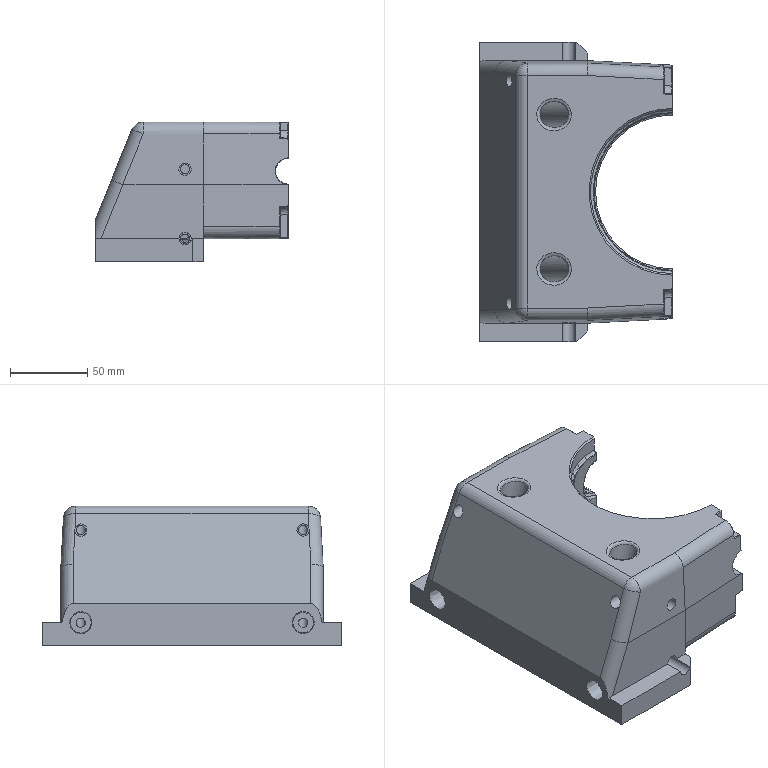Part | NX | features solid 2 | 1 solid | 326 faces | box 125 x 194 x 90.5 mm | volume 1235222 mm3 | plane 123 | spline 113 | cylinder 68 | cone 13 | sphere 6 | torus 3 | commonest cylinder face diameters 6 x25 8 x15 16 x11 10 x4 102.409 x4 26.633 x3